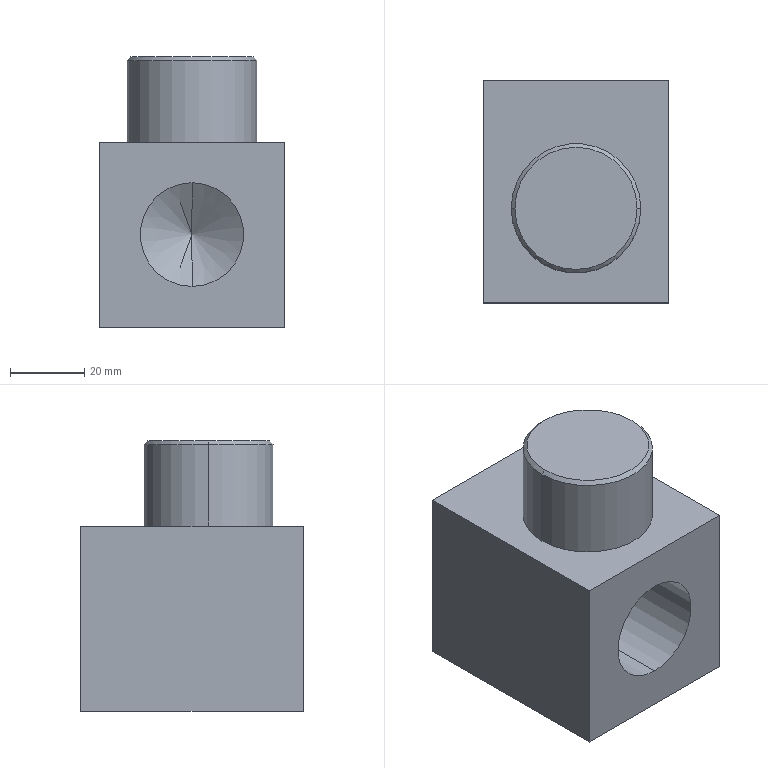Part | SolidWorks | features Chamfer 1, Extrusion 1, HoleWzd 1, ICE 1 | 1 solid | 15 faces | box 50 x 60 x 73 mm | volume 158033 mm3 | plane 7 | cone 4 | cylinder 4 | commonest cylinder face diameters 28 x2 35 x2
STEP:
#1=CARTESIAN_POINT('',(16.5,-4.5,73.));
#2=VERTEX_POINT('',#1);
#3=CARTESIAN_POINT('',(-16.5,-4.5,73.));
#4=VERTEX_POINT('',#3);
#5=CARTESIAN_POINT('',(0.,-4.5,73.));
#6=DIRECTION('',(0.,0.,1.));
#7=DIRECTION('',(1.,0.,0.));
#8=AXIS2_PLACEMENT_3D('',#5,#6,#7);
#9=CIRCLE('',#8,16.5);
#10=EDGE_CURVE('',#2,#4,#9,.T.);
#11=ORIENTED_EDGE('',*,*,#10,.F.);
#12=CARTESIAN_POINT('',(17.5,-4.5,72.));
#13=VERTEX_POINT('',#12);
#14=CARTESIAN_POINT('',(16.5,-4.5,73.));
#15=DIRECTION('',(0.7071,0.,-0.7071));
#16=VECTOR('',#15,1000.);
#17=LINE('',#14,#16);
#18=EDGE_CURVE('',#2,#13,#17,.T.);
#19=ORIENTED_EDGE('',*,*,#18,.T.);
#20=CARTESIAN_POINT('',(-17.5,-4.5,72.));
#21=VERTEX_POINT('',#20);
#22=CARTESIAN_POINT('',(0.,-4.5,72.));
#23=DIRECTION('',(0.,0.,-1.));
#24=DIRECTION('',(1.,0.,0.));
#25=AXIS2_PLACEMENT_3D('',#22,#23,#24);
#26=CIRCLE('',#25,17.5);
#27=EDGE_CURVE('',#21,#13,#26,.T.);
#28=ORIENTED_EDGE('',*,*,#27,.F.);
#29=CARTESIAN_POINT('',(-16.5,-4.5,73.));
#30=DIRECTION('',(-0.7071,0.,-0.7071));
#31=VECTOR('',#30,1000.);
#32=LINE('',#29,#31);
#33=EDGE_CURVE('',#4,#21,#32,.T.);
#34=ORIENTED_EDGE('',*,*,#33,.F.);
#35=EDGE_LOOP('',(#11,#19,#28,#34));
#36=FACE_OUTER_BOUND('',#35,.T.);
#37=CARTESIAN_POINT('',(0.,-4.5,73.));
#38=DIRECTION('',(0.,0.,-1.));
#39=DIRECTION('',(-1.,0.,0.));
#40=AXIS2_PLACEMENT_3D('',#37,#38,#39);
#41=CONICAL_SURFACE('',#40,16.5,0.7854);
#42=ADVANCED_FACE('',(#36),#41,.T.);
#43=CARTESIAN_POINT('',(0.,-10.,39.));
#44=VERTEX_POINT('',#43);
#45=CARTESIAN_POINT('',(0.,-10.,11.));
#46=VERTEX_POINT('',#45);
#47=CARTESIAN_POINT('',(0.,-10.,25.));
#48=DIRECTION('',(0.,-1.,0.));
#49=DIRECTION('',(0.,0.,-1.));
#50=AXIS2_PLACEMENT_3D('',#47,#48,#49);
#51=CIRCLE('',#50,14.);
#52=EDGE_CURVE('',#44,#46,#51,.T.);
#53=ORIENTED_EDGE('',*,*,#52,.F.);
#54=CARTESIAN_POINT('',(0.,-30.,39.));
#55=VERTEX_POINT('',#54);
#56=CARTESIAN_POINT('',(0.,-30.,39.));
#57=DIRECTION('',(0.,-1.,0.));
#58=VECTOR('',#57,1000.);
#59=LINE('',#56,#58);
#60=EDGE_CURVE('',#44,#55,#59,.T.);
#61=ORIENTED_EDGE('',*,*,#60,.T.);
#62=CARTESIAN_POINT('',(0.,-30.,11.));
#63=VERTEX_POINT('',#62);
#64=CARTESIAN_POINT('',(0.,-30.,25.));
#65=DIRECTION('',(0.,-1.,0.));
#66=DIRECTION('',(0.,0.,-1.));
#67=AXIS2_PLACEMENT_3D('',#64,#65,#66);
#68=CIRCLE('',#67,14.);
#69=EDGE_CURVE('',#55,#63,#68,.T.);
#70=ORIENTED_EDGE('',*,*,#69,.T.);
#71=CARTESIAN_POINT('',(0.,-30.,11.));
#72=DIRECTION('',(0.,-1.,0.));
#73=VECTOR('',#72,1000.);
#74=LINE('',#71,#73);
#75=EDGE_CURVE('',#46,#63,#74,.T.);
#76=ORIENTED_EDGE('',*,*,#75,.F.);
#77=EDGE_LOOP('',(#53,#61,#70,#76));
#78=FACE_OUTER_BOUND('',#77,.T.);
#79=CARTESIAN_POINT('',(0.,-30.,25.));
#80=DIRECTION('',(0.,-1.,0.));
#81=DIRECTION('',(0.,0.,-1.));
#82=AXIS2_PLACEMENT_3D('',#79,#80,#81);
#83=CYLINDRICAL_SURFACE('',#82,14.);
#84=ADVANCED_FACE('',(#78),#83,.F.);
#85=CARTESIAN_POINT('',(0.,-1.588,25.));
#86=VERTEX_POINT('',#85);
#87=CARTESIAN_POINT('',(0.,-10.,11.));
#88=DIRECTION('',(0.,-0.515,-0.8572));
#89=VECTOR('',#88,1000.);
#90=LINE('',#87,#89);
#91=EDGE_CURVE('',#86,#46,#90,.T.);
#92=ORIENTED_EDGE('',*,*,#91,.F.);
#93=CARTESIAN_POINT('',(0.,-10.,39.));
#94=DIRECTION('',(0.,-0.515,0.8572));
#95=VECTOR('',#94,1000.);
#96=LINE('',#93,#95);
#97=EDGE_CURVE('',#86,#44,#96,.T.);
#98=ORIENTED_EDGE('',*,*,#97,.T.);
#99=ORIENTED_EDGE('',*,*,#52,.T.);
#100=EDGE_LOOP('',(#92,#98,#99));
#101=FACE_OUTER_BOUND('',#100,.T.);
#102=CARTESIAN_POINT('',(0.,-10.,25.));
#103=DIRECTION('',(0.,-1.,0.));
#104=DIRECTION('',(0.,0.,-1.));
#105=AXIS2_PLACEMENT_3D('',#102,#103,#104);
#106=CONICAL_SURFACE('',#105,14.,1.03);
#107=ADVANCED_FACE('',(#101),#106,.F.);
#108=ORIENTED_EDGE('',*,*,#27,.T.);
#109=CARTESIAN_POINT('',(17.5,-4.5,50.));
#110=VERTEX_POINT('',#109);
#111=CARTESIAN_POINT('',(17.5,-4.5,73.));
#112=DIRECTION('',(0.,0.,-1.));
#113=VECTOR('',#112,1000.);
#114=LINE('',#111,#113);
#115=EDGE_CURVE('',#13,#110,#114,.T.);
#116=ORIENTED_EDGE('',*,*,#115,.T.);
#117=CARTESIAN_POINT('',(-17.5,-4.5,50.));
#118=VERTEX_POINT('',#117);
#119=CARTESIAN_POINT('',(0.,-4.5,50.));
#120=DIRECTION('',(0.,0.,1.));
#121=DIRECTION('',(1.,0.,0.));
#122=AXIS2_PLACEMENT_3D('',#119,#120,#121);
#123=CIRCLE('',#122,17.5);
#124=EDGE_CURVE('',#110,#118,#123,.T.);
#125=ORIENTED_EDGE('',*,*,#124,.T.);
#126=CARTESIAN_POINT('',(-17.5,-4.5,73.));
#127=DIRECTION('',(0.,0.,-1.));
#128=VECTOR('',#127,1000.);
#129=LINE('',#126,#128);
#130=EDGE_CURVE('',#21,#118,#129,.T.);
#131=ORIENTED_EDGE('',*,*,#130,.F.);
#132=EDGE_LOOP('',(#108,#116,#125,#131));
#133=FACE_OUTER_BOUND('',#132,.T.);
#134=CARTESIAN_POINT('',(0.,-4.5,73.));
#135=DIRECTION('',(0.,0.,-1.));
#136=DIRECTION('',(-1.,0.,0.));
#137=AXIS2_PLACEMENT_3D('',#134,#135,#136);
#138=CYLINDRICAL_SURFACE('',#137,17.5);
#139=ADVANCED_FACE('',(#133),#138,.T.);
#140=CARTESIAN_POINT('',(25.,-30.,0.));
#141=VERTEX_POINT('',#140);
#142=CARTESIAN_POINT('',(25.,30.,0.));
#143=VERTEX_POINT('',#142);
#144=CARTESIAN_POINT('',(25.,-30.,0.));
#145=DIRECTION('',(0.,1.,0.));
#146=VECTOR('',#145,1000.);
#147=LINE('',#144,#146);
#148=EDGE_CURVE('',#141,#143,#147,.T.);
#149=ORIENTED_EDGE('',*,*,#148,.T.);
#150=CARTESIAN_POINT('',(25.,30.,50.));
#151=VERTEX_POINT('',#150);
#152=CARTESIAN_POINT('',(25.,30.,50.));
#153=DIRECTION('',(0.,0.,-1.));
#154=VECTOR('',#153,1000.);
#155=LINE('',#152,#154);
#156=EDGE_CURVE('',#151,#143,#155,.T.);
#157=ORIENTED_EDGE('',*,*,#156,.F.);
#158=CARTESIAN_POINT('',(25.,-30.,50.));
#159=VERTEX_POINT('',#158);
#160=CARTESIAN_POINT('',(25.,-30.,50.));
#161=DIRECTION('',(0.,1.,0.));
#162=VECTOR('',#161,1000.);
#163=LINE('',#160,#162);
#164=EDGE_CURVE('',#159,#151,#163,.T.);
#165=ORIENTED_EDGE('',*,*,#164,.F.);
#166=CARTESIAN_POINT('',(25.,-30.,50.));
#167=DIRECTION('',(0.,0.,-1.));
#168=VECTOR('',#167,1000.);
#169=LINE('',#166,#168);
#170=EDGE_CURVE('',#159,#141,#169,.T.);
#171=ORIENTED_EDGE('',*,*,#170,.T.);
#172=EDGE_LOOP('',(#149,#157,#165,#171));
#173=FACE_OUTER_BOUND('',#172,.T.);
#174=CARTESIAN_POINT('',(25.,-30.,50.));
#175=DIRECTION('',(-1.,0.,0.));
#176=DIRECTION('',(0.,0.,1.));
#177=AXIS2_PLACEMENT_3D('',#174,#175,#176);
#178=PLANE('',#177);
#179=ADVANCED_FACE('',(#173),#178,.F.);
#180=CARTESIAN_POINT('',(-25.,30.,0.));
#181=VERTEX_POINT('',#180);
#182=CARTESIAN_POINT('',(-25.,30.,0.));
#183=DIRECTION('',(-1.,0.,0.));
#184=VECTOR('',#183,1000.);
#185=LINE('',#182,#184);
#186=EDGE_CURVE('',#143,#181,#185,.T.);
#187=ORIENTED_EDGE('',*,*,#186,.T.);
#188=CARTESIAN_POINT('',(-25.,30.,50.));
#189=VERTEX_POINT('',#188);
#190=CARTESIAN_POINT('',(-25.,30.,50.));
#191=DIRECTION('',(0.,0.,-1.));
#192=VECTOR('',#191,1000.);
#193=LINE('',#190,#192);
#194=EDGE_CURVE('',#189,#181,#193,.T.);
#195=ORIENTED_EDGE('',*,*,#194,.F.);
#196=CARTESIAN_POINT('',(-25.,30.,50.));
#197=DIRECTION('',(-1.,0.,0.));
#198=VECTOR('',#197,1000.);
#199=LINE('',#196,#198);
#200=EDGE_CURVE('',#151,#189,#199,.T.);
#201=ORIENTED_EDGE('',*,*,#200,.F.);
#202=ORIENTED_EDGE('',*,*,#156,.T.);
#203=EDGE_LOOP('',(#187,#195,#201,#202));
#204=FACE_OUTER_BOUND('',#203,.T.);
#205=CARTESIAN_POINT('',(-25.,30.,50.));
#206=DIRECTION('',(0.,-1.,0.));
#207=DIRECTION('',(0.,0.,-1.));
#208=AXIS2_PLACEMENT_3D('',#205,#206,#207);
#209=PLANE('',#208);
#210=ADVANCED_FACE('',(#204),#209,.F.);
#211=CARTESIAN_POINT('',(-25.,-30.,0.));
#212=VERTEX_POINT('',#211);
#213=CARTESIAN_POINT('',(-25.,-30.,0.));
#214=DIRECTION('',(0.,-1.,0.));
#215=VECTOR('',#214,1000.);
#216=LINE('',#213,#215);
#217=EDGE_CURVE('',#181,#212,#216,.T.);
#218=ORIENTED_EDGE('',*,*,#217,.T.);
#219=CARTESIAN_POINT('',(-25.,-30.,50.));
#220=VERTEX_POINT('',#219);
#221=CARTESIAN_POINT('',(-25.,-30.,50.));
#222=DIRECTION('',(0.,0.,-1.));
#223=VECTOR('',#222,1000.);
#224=LINE('',#221,#223);
#225=EDGE_CURVE('',#220,#212,#224,.T.);
#226=ORIENTED_EDGE('',*,*,#225,.F.);
#227=CARTESIAN_POINT('',(-25.,-30.,50.));
#228=DIRECTION('',(0.,-1.,0.));
#229=VECTOR('',#228,1000.);
#230=LINE('',#227,#229);
#231=EDGE_CURVE('',#189,#220,#230,.T.);
#232=ORIENTED_EDGE('',*,*,#231,.F.);
#233=ORIENTED_EDGE('',*,*,#194,.T.);
#234=EDGE_LOOP('',(#218,#226,#232,#233));
#235=FACE_OUTER_BOUND('',#234,.T.);
#236=CARTESIAN_POINT('',(-25.,-30.,50.));
#237=DIRECTION('',(1.,0.,0.));
#238=DIRECTION('',(0.,0.,-1.));
#239=AXIS2_PLACEMENT_3D('',#236,#237,#238);
#240=PLANE('',#239);
#241=ADVANCED_FACE('',(#235),#240,.F.);
#242=CARTESIAN_POINT('',(0.,-30.,25.));
#243=DIRECTION('',(0.,-1.,0.));
#244=DIRECTION('',(0.,0.,-1.));
#245=AXIS2_PLACEMENT_3D('',#242,#243,#244);
#246=CIRCLE('',#245,14.);
#247=EDGE_CURVE('',#63,#55,#246,.T.);
#248=ORIENTED_EDGE('',*,*,#247,.F.);
#249=ORIENTED_EDGE('',*,*,#69,.F.);
#250=EDGE_LOOP('',(#248,#249));
#251=FACE_BOUND('',#250,.T.);
#252=CARTESIAN_POINT('',(-25.,-30.,0.));
#253=DIRECTION('',(1.,0.,0.));
#254=VECTOR('',#253,1000.);
#255=LINE('',#252,#254);
#256=EDGE_CURVE('',#212,#141,#255,.T.);
#257=ORIENTED_EDGE('',*,*,#256,.T.);
#258=ORIENTED_EDGE('',*,*,#170,.F.);
#259=CARTESIAN_POINT('',(-25.,-30.,50.));
#260=DIRECTION('',(1.,0.,0.));
#261=VECTOR('',#260,1000.);
#262=LINE('',#259,#261);
#263=EDGE_CURVE('',#220,#159,#262,.T.);
#264=ORIENTED_EDGE('',*,*,#263,.F.);
#265=ORIENTED_EDGE('',*,*,#225,.T.);
#266=EDGE_LOOP('',(#257,#258,#264,#265));
#267=FACE_OUTER_BOUND('',#266,.T.);
#268=CARTESIAN_POINT('',(-25.,-30.,50.));
#269=DIRECTION('',(0.,1.,0.));
#270=DIRECTION('',(0.,0.,1.));
#271=AXIS2_PLACEMENT_3D('',#268,#269,#270);
#272=PLANE('',#271);
#273=ADVANCED_FACE('',(#251,#267),#272,.F.);
#274=CARTESIAN_POINT('',(0.,-4.5,50.));
#275=DIRECTION('',(0.,0.,1.));
#276=DIRECTION('',(1.,0.,0.));
#277=AXIS2_PLACEMENT_3D('',#274,#275,#276);
#278=CIRCLE('',#277,17.5);
#279=EDGE_CURVE('',#118,#110,#278,.T.);
#280=ORIENTED_EDGE('',*,*,#279,.F.);
#281=ORIENTED_EDGE('',*,*,#124,.F.);
#282=EDGE_LOOP('',(#280,#281));
#283=FACE_BOUND('',#282,.T.);
#284=ORIENTED_EDGE('',*,*,#164,.T.);
#285=ORIENTED_EDGE('',*,*,#200,.T.);
#286=ORIENTED_EDGE('',*,*,#231,.T.);
#287=ORIENTED_EDGE('',*,*,#263,.T.);
#288=EDGE_LOOP('',(#284,#285,#286,#287));
#289=FACE_OUTER_BOUND('',#288,.T.);
#290=CARTESIAN_POINT('',(0.,0.,50.));
#291=DIRECTION('',(0.,0.,-1.));
#292=DIRECTION('',(-1.,0.,0.));
#293=AXIS2_PLACEMENT_3D('',#290,#291,#292);
#294=PLANE('',#293);
#295=ADVANCED_FACE('',(#283,#289),#294,.F.);
#296=ORIENTED_EDGE('',*,*,#148,.F.);
#297=ORIENTED_EDGE('',*,*,#256,.F.);
#298=ORIENTED_EDGE('',*,*,#217,.F.);
#299=ORIENTED_EDGE('',*,*,#186,.F.);
#300=EDGE_LOOP('',(#296,#297,#298,#299));
#301=FACE_OUTER_BOUND('',#300,.T.);
#302=CARTESIAN_POINT('',(0.,0.,0.));
#303=DIRECTION('',(0.,0.,-1.));
#304=DIRECTION('',(-1.,0.,0.));
#305=AXIS2_PLACEMENT_3D('',#302,#303,#304);
#306=PLANE('',#305);
#307=ADVANCED_FACE('',(#301),#306,.T.);
#308=ORIENTED_EDGE('',*,*,#115,.F.);
#309=CARTESIAN_POINT('',(0.,-4.5,72.));
#310=DIRECTION('',(0.,0.,-1.));
#311=DIRECTION('',(1.,0.,0.));
#312=AXIS2_PLACEMENT_3D('',#309,#310,#311);
#313=CIRCLE('',#312,17.5);
#314=EDGE_CURVE('',#13,#21,#313,.T.);
#315=ORIENTED_EDGE('',*,*,#314,.T.);
#316=ORIENTED_EDGE('',*,*,#130,.T.);
#317=ORIENTED_EDGE('',*,*,#279,.T.);
#318=EDGE_LOOP('',(#308,#315,#316,#317));
#319=FACE_OUTER_BOUND('',#318,.T.);
#320=CARTESIAN_POINT('',(0.,-4.5,73.));
#321=DIRECTION('',(0.,0.,-1.));
#322=DIRECTION('',(-1.,0.,0.));
#323=AXIS2_PLACEMENT_3D('',#320,#321,#322);
#324=CYLINDRICAL_SURFACE('',#323,17.5);
#325=ADVANCED_FACE('',(#319),#324,.T.);
#326=CARTESIAN_POINT('',(0.,-4.5,73.));
#327=DIRECTION('',(0.,0.,1.));
#328=DIRECTION('',(1.,0.,0.));
#329=AXIS2_PLACEMENT_3D('',#326,#327,#328);
#330=CIRCLE('',#329,16.5);
#331=EDGE_CURVE('',#4,#2,#330,.T.);
#332=ORIENTED_EDGE('',*,*,#331,.T.);
#333=ORIENTED_EDGE('',*,*,#10,.T.);
#334=EDGE_LOOP('',(#332,#333));
#335=FACE_OUTER_BOUND('',#334,.T.);
#336=CARTESIAN_POINT('',(0.,-4.5,73.));
#337=DIRECTION('',(0.,0.,1.));
#338=DIRECTION('',(1.,0.,0.));
#339=AXIS2_PLACEMENT_3D('',#336,#337,#338);
#340=PLANE('',#339);
#341=ADVANCED_FACE('',(#335),#340,.T.);
#342=ORIENTED_EDGE('',*,*,#97,.F.);
#343=ORIENTED_EDGE('',*,*,#91,.T.);
#344=CARTESIAN_POINT('',(0.,-10.,25.));
#345=DIRECTION('',(0.,-1.,0.));
#346=DIRECTION('',(0.,0.,-1.));
#347=AXIS2_PLACEMENT_3D('',#344,#345,#346);
#348=CIRCLE('',#347,14.);
#349=EDGE_CURVE('',#46,#44,#348,.T.);
#350=ORIENTED_EDGE('',*,*,#349,.T.);
#351=EDGE_LOOP('',(#342,#343,#350));
#352=FACE_OUTER_BOUND('',#351,.T.);
#353=CARTESIAN_POINT('',(0.,-10.,25.));
#354=DIRECTION('',(0.,-1.,0.));
#355=DIRECTION('',(0.,0.,-1.));
#356=AXIS2_PLACEMENT_3D('',#353,#354,#355);
#357=CONICAL_SURFACE('',#356,14.,1.03);
#358=ADVANCED_FACE('',(#352),#357,.F.);
#359=ORIENTED_EDGE('',*,*,#60,.F.);
#360=ORIENTED_EDGE('',*,*,#349,.F.);
#361=ORIENTED_EDGE('',*,*,#75,.T.);
#362=ORIENTED_EDGE('',*,*,#247,.T.);
#363=EDGE_LOOP('',(#359,#360,#361,#362));
#364=FACE_OUTER_BOUND('',#363,.T.);
#365=CARTESIAN_POINT('',(0.,-30.,25.));
#366=DIRECTION('',(0.,-1.,0.));
#367=DIRECTION('',(0.,0.,-1.));
#368=AXIS2_PLACEMENT_3D('',#365,#366,#367);
#369=CYLINDRICAL_SURFACE('',#368,14.);
#370=ADVANCED_FACE('',(#364),#369,.F.);
#371=ORIENTED_EDGE('',*,*,#18,.F.);
#372=ORIENTED_EDGE('',*,*,#331,.F.);
#373=ORIENTED_EDGE('',*,*,#33,.T.);
#374=ORIENTED_EDGE('',*,*,#314,.F.);
#375=EDGE_LOOP('',(#371,#372,#373,#374));
#376=FACE_OUTER_BOUND('',#375,.T.);
#377=CARTESIAN_POINT('',(0.,-4.5,73.));
#378=DIRECTION('',(0.,0.,-1.));
#379=DIRECTION('',(-1.,0.,0.));
#380=AXIS2_PLACEMENT_3D('',#377,#378,#379);
#381=CONICAL_SURFACE('',#380,16.5,0.7854);
#382=ADVANCED_FACE('',(#376),#381,.T.);
#383=CLOSED_SHELL('',(#42,#84,#107,#139,#179,#210,#241,#273,#295,#307,#325,#341,#358,#370,#382));
#384=MANIFOLD_SOLID_BREP('',#383);
#385=CARTESIAN_POINT('',(0.,0.,0.));
#386=DIRECTION('',(0.,0.,1.));
#387=DIRECTION('',(1.,0.,0.));
#388=AXIS2_PLACEMENT_3D('',#385,#386,#387);
#389=(LENGTH_UNIT()NAMED_UNIT(*)SI_UNIT(.MILLI.,.METRE.));
#390=UNCERTAINTY_MEASURE_WITH_UNIT(LENGTH_MEASURE(0.00001),#389,'','');
#391=(NAMED_UNIT(*)PLANE_ANGLE_UNIT()SI_UNIT($,.RADIAN.));
#392=(NAMED_UNIT(*)SI_UNIT($,.STERADIAN.)SOLID_ANGLE_UNIT());
#393=(GEOMETRIC_REPRESENTATION_CONTEXT(3)GLOBAL_UNCERTAINTY_ASSIGNED_CONTEXT((#390))GLOBAL_UNIT_ASSIGNED_CONTEXT((#389,#391,#392))REPRESENTATION_CONTEXT('',''));
#394=ADVANCED_BREP_SHAPE_REPRESENTATION('',(#384,#388),#393);